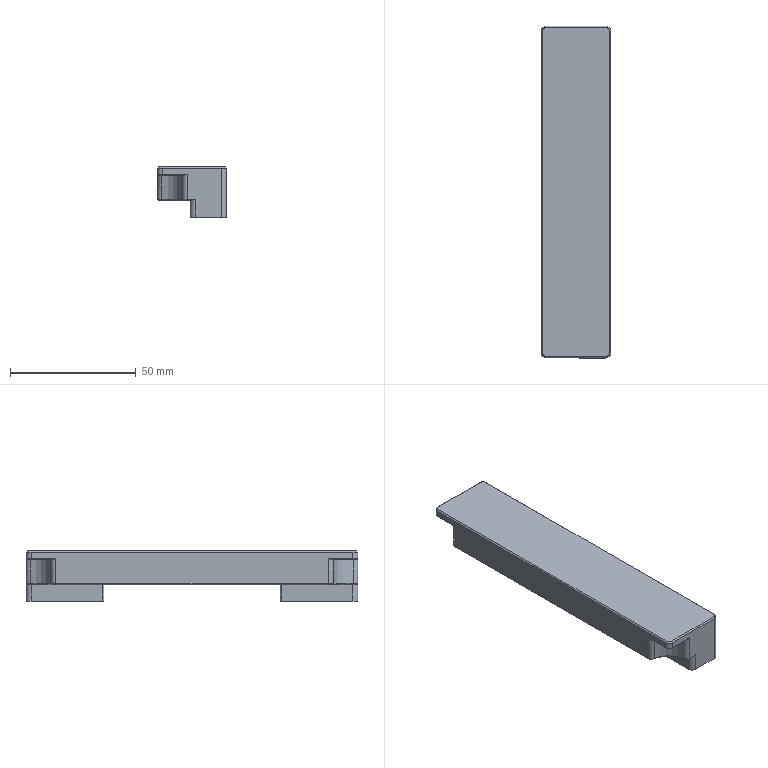NC program | NX | posted with a generic post | part box 27.5 x 132 x 20 mm
Lines 1924 to 2947 of 2947:
(ZLEVEL_PROFILE_COPY_1_COPY , TOOL : D10JING)
N3822 T14 M6
N3824 G54
N3826 G17 G0 G90 X45.895 Y-18.75 S9500 M3
N3828 G43 Z30. H14
N3830 Z1.5
N3832 G94 G1 X-64.649 Z-4.293 F1000.
N3834 X-66.234 Y-18.416 Z-4.378
N3836 X-67.701 Y-17.727 Z-4.463
N3838 X-68.971 Y-16.721 Z-4.548
N3840 X-69.977 Y-15.451 Z-4.633
N3842 X-70.666 Y-13.984 Z-4.718
N3844 X-71. Y-12.399 Z-4.803
N3846 Y12.399 Z-6.102
N3848 X-70.666 Y13.984 Z-6.187
N3850 X-69.977 Y15.451 Z-6.272
N3852 X-68.971 Y16.721 Z-6.357
N3854 X-67.701 Y17.727 Z-6.442
N3856 X-66.234 Y18.416 Z-6.527
N3858 X-64.649 Y18.75 Z-6.612
N3860 X0. Z-10.
N3862 X64. F1200.
N3864 G2 X71. Y11.75 R7.
N3866 G1 Y-11.75
N3868 G2 X64. Y-18.75 R7.
N3870 G1 X-64.
N3872 G2 X-71. Y-11.75 R7.
N3874 G1 Y11.75
N3876 G2 X-64. Y18.75 R7.
N3878 G1 X0.
N3880 X64. Z-11.845
N3882 X64.61 Y18.723 Z-11.862
N3884 X65.216 Y18.644 Z-11.88
N3886 X65.812 Y18.511 Z-11.898
N3888 X66.394 Y18.328 Z-11.915
N3890 X66.958 Y18.094 Z-11.933
N3892 X67.5 Y17.812 Z-11.95
N3894 X68.015 Y17.484 Z-11.968
N3896 X68.5 Y17.112 Z-11.985
N3898 X68.95 Y16.7 Z-12.003
N3900 X69.362 Y16.25 Z-12.021
N3902 X69.734 Y15.765 Z-12.038
N3904 X70.062 Y15.25 Z-12.056
N3906 X70.344 Y14.708 Z-12.073
N3908 X70.578 Y14.144 Z-12.091
N3910 X70.761 Y13.562 Z-12.109
N3912 X70.894 Y12.966 Z-12.126
N3914 X70.973 Y12.36 Z-12.144
N3916 X71. Y11.75 Z-12.161
N3918 Y-11.75 Z-12.839
N3920 X70.973 Y-12.36 Z-12.856
N3922 X70.894 Y-12.966 Z-12.874
N3924 X70.761 Y-13.562 Z-12.891
N3926 X70.578 Y-14.144 Z-12.909
N3928 X70.344 Y-14.708 Z-12.927
N3930 X70.062 Y-15.25 Z-12.944
N3932 X69.734 Y-15.765 Z-12.962
N3934 X69.362 Y-16.25 Z-12.979
N3936 X68.95 Y-16.7 Z-12.997
N3938 X68.5 Y-17.112 Z-13.015
N3940 X68.015 Y-17.484 Z-13.032
N3942 X67.5 Y-17.812 Z-13.05
N3944 X66.958 Y-18.094 Z-13.067
N3946 X66.394 Y-18.328 Z-13.085
N3948 X65.812 Y-18.511 Z-13.102
N3950 X65.216 Y-18.644 Z-13.12
N3952 X64.61 Y-18.723 Z-13.138
N3954 X64. Y-18.75 Z-13.155
N3956 X-64. Z-16.845
N3958 X-64.61 Y-18.723 Z-16.862
N3960 X-65.216 Y-18.644 Z-16.88
N3962 X-65.812 Y-18.511 Z-16.898
N3964 X-66.394 Y-18.328 Z-16.915
N3966 X-66.958 Y-18.094 Z-16.933
N3968 X-67.5 Y-17.812 Z-16.95
N3970 X-68.015 Y-17.484 Z-16.968
N3972 X-68.5 Y-17.112 Z-16.985
N3974 X-68.95 Y-16.7 Z-17.003
N3976 X-69.362 Y-16.25 Z-17.021
N3978 X-69.734 Y-15.765 Z-17.038
N3980 X-70.062 Y-15.25 Z-17.056
N3982 X-70.344 Y-14.708 Z-17.073
N3984 X-70.578 Y-14.144 Z-17.091
N3986 X-70.761 Y-13.562 Z-17.109
N3988 X-70.894 Y-12.966 Z-17.126
N3990 X-70.973 Y-12.36 Z-17.144
N3992 X-71. Y-11.75 Z-17.161
N3994 Y11.75 Z-17.839
N3996 X-70.973 Y12.36 Z-17.856
N3998 X-70.894 Y12.966 Z-17.874
N4000 X-70.761 Y13.562 Z-17.891
N4002 X-70.578 Y14.144 Z-17.909
N4004 X-70.344 Y14.708 Z-17.927
N4006 X-70.062 Y15.25 Z-17.944
N4008 X-69.734 Y15.765 Z-17.962
N4010 X-69.362 Y16.25 Z-17.979
N4012 X-68.95 Y16.7 Z-17.997
N4014 X-68.5 Y17.112 Z-18.015
N4016 X-68.015 Y17.484 Z-18.032
N4018 X-67.5 Y17.812 Z-18.05
N4020 X-66.958 Y18.094 Z-18.067
N4022 X-66.394 Y18.328 Z-18.085
N4024 X-65.812 Y18.511 Z-18.102
N4026 X-65.216 Y18.644 Z-18.12
N4028 X-64.61 Y18.723 Z-18.138
N4030 X-64. Y18.75 Z-18.155
N4032 X0. Z-20.
N4034 X64.
N4036 G2 X71. Y11.75 R7.
N4038 G1 Y-11.75
N4040 G2 X64. Y-18.75 R7.
N4042 G1 X-64.
N4044 G2 X-71. Y-11.75 R7.
N4046 G1 Y11.75
N4048 G2 X-64. Y18.75 R7.
N4050 G1 X0.
N4052 G3 X0.866 Y19.25 R1.
N4054 G1 X1.155 Y19.75
N4056 Z-19.
N4058 G0 Z30.
(FLOOR_WALL_2 , TOOL : D10JING)
N4060 X-73.846 Y-3.664
N4062 Z-13.5
N4064 G1 Z-16.5 F1500.
N4066 X-70.5 Y-5.715
N4068 X-70.45 Y-5.746
N4070 G3 X-65.25 Y-9.313 R7.5
N4072 G2 X-63.649 Y-9.913 R4.5
N4074 G1 X-63.648 Z-13.5
N4076 G0 Z30.
N4078 X-54.067 Y-21.75
N4080 Z-13.5
N4082 G1 Z-16.5
N4084 Y-19.365
N4086 X-56.84 Y-18.22
N4088 G2 X-61.07 Y-12.917 R7.
N4090 G3 X-65.167 Y-8.82 R5.
N4092 G2 X-70.47 Y-4.59 R7.
N4094 G1 X-71.615 Y-1.817
N4096 X-74.
N4098 Z-13.5
N4100 G0 Z30.
N4102 X-27. Y7.25
N4104 Z-3.5
N4106 G1 Z-6.5
N4108 X-29.5 Y4.25
N4110 X29.5
N4112 Y-0.25
N4114 X-29.5
N4116 Y-2.321
N4118 G2 X-29.646 Y-2.675 R0.5
N4120 G1 X-31.722 Y-4.75
N4122 X31.722
N4124 X33.075 Y-6.104
N4126 G3 X33.429 Y-6.25 R0.5
N4128 G1 X64.
N4130 G3 X68.5 Y-4.75 R7.5
N4132 G1 X69.851
N4134 X73.068
N4136 Z-3.5
N4138 G0 Z30.
N4140 X-73.068
N4142 Z-3.5
N4144 G1 Z-6.5
N4146 X-69.851
N4148 X-68.5
N4150 X-72.04 Y-6.978
N4152 Z-3.5
N4154 G0 Z30.
N4156 X70.041 Y-9.25
N4158 Z-3.5
N4160 G1 Z-6.5
N4162 X62.838
N4164 X-62.838
N4166 X-70.041
N4168 Z-3.5
N4170 G0 Z30.
N4172 X-27. Y7.25
N4174 Z-3.5
N4176 G1 Z-6.5
N4178 X-30.
N4180 Y4.25
N4182 Y-2.321
N4184 X-33.429 Y-5.75
N4186 X-64.
N4188 G2 X-70.47 Y-1.422 R7.
N4190 G1 X-71.615 Y1.351
N4192 X-74.
N4194 Z-3.5
N4196 G0 Z30.
N4198 X74.
N4200 Z-3.5
N4202 G1 Z-6.5
N4204 X71.615
N4206 X70.47 Y-1.422
N4208 G2 X64. Y-5.75 R7.
N4210 G1 X33.429
N4212 X30. Y-2.321
N4214 Y4.25
N4216 Y7.25
N4218 X27.
N4220 Z-3.5
N4222 G0 Z30.
N4224 X-34.307 Y21.75
N4226 Z-13.5
N4228 G1 Z-16.5
N4230 Y18.75
N4232 X34.307
N4234 G3 X29.872 Y14.083 R7.5
N4236 G1 X-29.872
N4238 G2 X-29.5 Y11.75 R7.5
N4240 G1 Y9.417
N4242 X29.5
N4244 Y4.75
N4246 X-29.5
N4248 Z-13.5
N4250 G0 Z30.
N4252 X-39.34 Y21.75
N4254 Z-13.5
N4256 G1 Z-16.5
N4258 Y18.997
N4260 X-36.353 Y18.72
N4262 G2 X-30. Y11.75 R7.
N4264 G1 Y4.25
N4266 X30.
N4268 Y11.75
N4270 G2 X36.353 Y18.72 R7.
N4272 G1 X39.34 Y18.997
N4274 Y21.75
N4276 Z-13.5
N4278 G0 Z30.
N4280 X73.5 Y-8.364
N4282 Z-13.5
N4284 G1 Z-16.5
N4286 X67.834
N4288 X61.776 Y-18.25
N4290 X57.965
N4292 X57.996 Y-18.2
N4294 Y-21.25
N4296 Z-13.5
N4298 G0 Z30.
N4300 Y-18.2
N4302 Z-13.5
N4304 G1 Z-16.5
N4306 G3 X61.563 Y-13. R7.5
N4308 G2 X62.16 Y-11.404 R4.5
N4310 G1 X62.166 Y-11.394
N4312 Z-13.5
N4314 G0 Z30.
N4316 X74. Y-1.817
N4318 Z-13.5
N4320 G1 Z-16.5
N4322 X71.615
N4324 X70.47 Y-4.59
N4326 G2 X65.167 Y-8.82 R7.
N4328 G3 X61.07 Y-12.917 R5.
N4330 G2 X56.84 Y-18.22 R7.
N4332 G1 X54.067 Y-19.365
N4334 Y-21.75
N4336 Z-13.5
N4338 G0 Z30.
N4340 M5
(HOLE_MILLING , TOOL : D4)
N4342 T11 M6
N4344 G54
N4346 G17 G0 G90 X-60. Y8.75 S9500 M3
N4348 G43 Z30. H11
N4350 Z0.5
N4352 G94 G3 X-59.5 Y9.25 R0.5 F1250.
N4354 X-60. Y9.75 R0.5
N4356 X-60. Y9.75 Z0.1 I0. J-1.
N4358 X-60. Y9.75 Z-0.3 I0. J-1.
N4360 X-60. Y9.75 Z-0.7 I0. J-1.
N4362 X-60. Y9.75 Z-1.1 I0. J-1.
N4364 X-60. Y9.75 Z-1.5 I0. J-1.
N4366 X-60. Y9.75 Z-1.9 I0. J-1.
N4368 X-60. Y9.75 Z-2.3 I0. J-1.
N4370 X-60. Y9.75 Z-2.7 I0. J-1.
N4372 X-60. Y9.75 Z-3.1 I0. J-1.
N4374 X-60. Y9.75 Z-3.5 I0. J-1.
N4376 X-60. Y9.75 Z-3.9 I0. J-1.
N4378 X-60. Y9.75 Z-4.3 I0. J-1.
N4380 X-60. Y9.75 Z-4.7 I0. J-1.
N4382 X-60. Y9.75 Z-5.1 I0. J-1.
N4384 X-60. Y9.75 Z-5.5 I0. J-1.
N4386 X-60. Y9.75 Z-5.9 I0. J-1.
N4388 X-60. Y9.75 Z-6.3 I0. J-1.
N4390 X-60. Y9.75 Z-6.7 I0. J-1.
N4392 X-60. Y9.75 Z-7.1 I0. J-1.
N4394 X-60. Y9.75 Z-7.5 I0. J-1.
N4396 X-60. Y9.75 Z-7.9 I0. J-1.
N4398 X-60. Y9.75 Z-8.3 I0. J-1.
N4400 X-60. Y9.75 Z-8.7 I0. J-1.
N4402 X-60. Y9.75 Z-9.1 I0. J-1.
N4404 X-60. Y9.75 Z-9.5 I0. J-1.
N4406 X-60. Y9.75 Z-9.9 I0. J-1.
N4408 X-60. Y9.75 Z-10.3 I0. J-1.
N4410 X-60. Y9.75 Z-10.7 I0. J-1.
N4412 X-60. Y9.75 Z-11.1 I0. J-1.
N4414 X-60. Y9.75 Z-11.5 I0. J-1.
N4416 X-60. Y9.75 Z-11.9 I0. J-1.
N4418 X-61. Y8.75 Z-12. R1.
N4420 X-60. Y7.75 R1.
N4422 X-61. Y8.75 R-1.
N4424 X-60.5 Y8.25 R0.5
N4426 X-60. Y8.75 R0.5
N4428 G0 Z30.
N4430 X-37.5 Y-8.75
N4432 Z-6.
N4434 G3 X-37. Y-8.25 R0.5
N4436 X-37.5 Y-7.75 R0.5
N4438 X-37.5 Y-7.75 Z-6.4 I0. J-1.
N4440 X-37.5 Y-7.75 Z-6.8 I0. J-1.
N4442 X-37.5 Y-7.75 Z-7.2 I0. J-1.
N4444 X-37.5 Y-7.75 Z-7.6 I0. J-1.
N4446 X-37.5 Y-7.75 Z-8. I0. J-1.
N4448 X-37.5 Y-7.75 Z-8.4 I0. J-1.
N4450 X-37.5 Y-7.75 Z-8.8 I0. J-1.
N4452 X-37.5 Y-7.75 Z-9.2 I0. J-1.
N4454 X-37.5 Y-7.75 Z-9.6 I0. J-1.
N4456 X-37.5 Y-7.75 Z-10. I0. J-1.
N4458 X-37.5 Y-7.75 Z-10.4 I0. J-1.
N4460 X-37.5 Y-7.75 Z-10.8 I0. J-1.
N4462 X-37.5 Y-7.75 Z-11.2 I0. J-1.
N4464 X-37.5 Y-7.75 Z-11.6 I0. J-1.
N4466 X-37.5 Y-7.75 Z-12. I0. J-1.
N4468 X-37.5 Y-7.75 Z-12.4 I0. J-1.
N4470 X-37.5 Y-7.75 Z-12.8 I0. J-1.
N4472 X-37.5 Y-7.75 Z-13.2 I0. J-1.
N4474 X-37.5 Y-7.75 Z-13.6 I0. J-1.
N4476 X-37.5 Y-7.75 Z-14. I0. J-1.
N4478 X-37.5 Y-7.75 Z-14.4 I0. J-1.
N4480 X-37.5 Y-7.75 Z-14.8 I0. J-1.
N4482 X-37.5 Y-7.75 Z-15.2 I0. J-1.
N4484 X-37.5 Y-7.75 Z-15.6 I0. J-1.
N4486 X-37.5 Y-7.75 Z-16. I0. J-1.
N4488 X-37.5 Y-7.75 Z-16.4 I0. J-1.
N4490 X-37.5 Y-7.75 Z-16.8 I0. J-1.
N4492 X-37.5 Y-9.75 Z-17. I0. J-1.
N4494 X-36.5 Y-8.75 R1.
N4496 X-37.5 Y-9.75 R-1.
N4498 X-37. Y-9.25 R0.5
N4500 X-37.5 Y-8.75 R0.5
N4502 G0 Z30.
N4504 X37.5
N4506 Z-6.
N4508 G3 X38. Y-8.25 R0.5
N4510 X37.5 Y-7.75 R0.5
N4512 X37.5 Y-7.75 Z-6.4 I0. J-1.
N4514 X37.5 Y-7.75 Z-6.8 I0. J-1.
N4516 X37.5 Y-7.75 Z-7.2 I0. J-1.
N4518 X37.5 Y-7.75 Z-7.6 I0. J-1.
N4520 X37.5 Y-7.75 Z-8. I0. J-1.
N4522 X37.5 Y-7.75 Z-8.4 I0. J-1.
N4524 X37.5 Y-7.75 Z-8.8 I0. J-1.
N4526 X37.5 Y-7.75 Z-9.2 I0. J-1.
N4528 X37.5 Y-7.75 Z-9.6 I0. J-1.
N4530 X37.5 Y-7.75 Z-10. I0. J-1.
N4532 X37.5 Y-7.75 Z-10.4 I0. J-1.
N4534 X37.5 Y-7.75 Z-10.8 I0. J-1.
N4536 X37.5 Y-7.75 Z-11.2 I0. J-1.
N4538 X37.5 Y-7.75 Z-11.6 I0. J-1.
N4540 X37.5 Y-7.75 Z-12. I0. J-1.
N4542 X37.5 Y-7.75 Z-12.4 I0. J-1.
N4544 X37.5 Y-7.75 Z-12.8 I0. J-1.
N4546 X37.5 Y-7.75 Z-13.2 I0. J-1.
N4548 X37.5 Y-7.75 Z-13.6 I0. J-1.
N4550 X37.5 Y-7.75 Z-14. I0. J-1.
N4552 X37.5 Y-7.75 Z-14.4 I0. J-1.
N4554 X37.5 Y-7.75 Z-14.8 I0. J-1.
N4556 X37.5 Y-7.75 Z-15.2 I0. J-1.
N4558 X37.5 Y-7.75 Z-15.6 I0. J-1.
N4560 X37.5 Y-7.75 Z-16. I0. J-1.
N4562 X37.5 Y-7.75 Z-16.4 I0. J-1.
N4564 X37.5 Y-7.75 Z-16.8 I0. J-1.
N4566 X37.5 Y-9.75 Z-17. I0. J-1.
N4568 X38.5 Y-8.75 R1.
N4570 X37.5 Y-9.75 R-1.
N4572 X38. Y-9.25 R0.5
N4574 X37.5 Y-8.75 R0.5
N4576 G0 Z30.
N4578 X60. Y8.75
N4580 Z0.5
N4582 G3 X60.5 Y9.25 R0.5
N4584 X60. Y9.75 R0.5
N4586 X60. Y9.75 Z0.1 I0. J-1.
N4588 X60. Y9.75 Z-0.3 I0. J-1.
N4590 X60. Y9.75 Z-0.7 I0. J-1.
N4592 X60. Y9.75 Z-1.1 I0. J-1.
N4594 X60. Y9.75 Z-1.5 I0. J-1.
N4596 X60. Y9.75 Z-1.9 I0. J-1.
N4598 X60. Y9.75 Z-2.3 I0. J-1.
N4600 X60. Y9.75 Z-2.7 I0. J-1.
N4602 X60. Y9.75 Z-3.1 I0. J-1.
N4604 X60. Y9.75 Z-3.5 I0. J-1.
N4606 X60. Y9.75 Z-3.9 I0. J-1.
N4608 X60. Y9.75 Z-4.3 I0. J-1.
N4610 X60. Y9.75 Z-4.7 I0. J-1.
N4612 X60. Y9.75 Z-5.1 I0. J-1.
N4614 X60. Y9.75 Z-5.5 I0. J-1.
N4616 X60. Y9.75 Z-5.9 I0. J-1.
N4618 X60. Y9.75 Z-6.3 I0. J-1.
N4620 X60. Y9.75 Z-6.7 I0. J-1.
N4622 X60. Y9.75 Z-7.1 I0. J-1.
N4624 X60. Y9.75 Z-7.5 I0. J-1.
N4626 X60. Y9.75 Z-7.9 I0. J-1.
N4628 X60. Y9.75 Z-8.3 I0. J-1.
N4630 X60. Y9.75 Z-8.7 I0. J-1.
N4632 X60. Y9.75 Z-9.1 I0. J-1.
N4634 X60. Y9.75 Z-9.5 I0. J-1.
N4636 X60. Y9.75 Z-9.9 I0. J-1.
N4638 X60. Y9.75 Z-10.3 I0. J-1.
N4640 X60. Y9.75 Z-10.7 I0. J-1.
N4642 X60. Y9.75 Z-11.1 I0. J-1.
N4644 X60. Y9.75 Z-11.5 I0. J-1.
N4646 X60. Y9.75 Z-11.9 I0. J-1.
N4648 X59. Y8.75 Z-12. R1.
N4650 X60. Y7.75 R1.
N4652 X59. Y8.75 R-1.
N4654 X59.5 Y8.25 R0.5
N4656 X60. Y8.75 R0.5
N4658 G0 Z30.
(ZLEVEL_PROFILE_COPY_1_COPY_1 , TOOL : D4)
N4660 X-32.6 Y4.609
N4662 Z-6.9
N4664 G1 X-32.8 Y4.493 F1000.
N4666 G3 X-33. Y4.147 R0.4
N4668 G1 Y1.25 F1800.
N4670 X-30.103
N4672 G3 X-29.757 Y1.45 R0.4
N4674 G1 X-29.641 Y1.65
N4676 G0 X-32.6 Y4.609 Z-7.3
N4678 G1 X-32.8 Y4.493 F1000.
N4680 G3 X-33. Y4.147 R0.4
N4682 G1 Y1.25 F1800.
N4684 X-30.103
N4686 G3 X-29.757 Y1.45 R0.4
N4688 G1 X-29.641 Y1.65
N4690 G0 X-32.6 Y4.609 Z-7.7
N4692 G1 X-32.8 Y4.493 F1000.
N4694 G3 X-33. Y4.147 R0.4
N4696 G1 Y1.25 F1800.
N4698 X-30.103
N4700 G3 X-29.757 Y1.45 R0.4
N4702 G1 X-29.641 Y1.65
N4704 G0 X-32.6 Y4.609 Z-8.1
N4706 G1 X-32.8 Y4.493 F1000.
N4708 G3 X-33. Y4.147 R0.4
N4710 G1 Y1.25 F1800.
N4712 X-30.103
N4714 G3 X-29.757 Y1.45 R0.4
N4716 G1 X-29.641 Y1.65
N4718 G0 X-32.6 Y4.609 Z-8.5
N4720 G1 X-32.8 Y4.493 F1000.
N4722 G3 X-33. Y4.147 R0.4
N4724 G1 Y1.25 F1800.
N4726 X-30.103
N4728 G3 X-29.757 Y1.45 R0.4
N4730 G1 X-29.641 Y1.65
N4732 G0 X-32.6 Y4.609 Z-8.9
N4734 G1 X-32.8 Y4.493 F1000.
N4736 G3 X-33. Y4.147 R0.4
N4738 G1 Y1.25 F1800.
N4740 X-30.103
N4742 G3 X-29.757 Y1.45 R0.4
N4744 G1 X-29.641 Y1.65
N4746 G0 X-32.6 Y4.609 Z-9.3
N4748 G1 X-32.8 Y4.493 F1000.
N4750 G3 X-33. Y4.147 R0.4
N4752 G1 Y1.25 F1800.
N4754 X-30.103
N4756 G3 X-29.757 Y1.45 R0.4
N4758 G1 X-29.641 Y1.65
N4760 G0 X-32.6 Y4.609 Z-9.7
N4762 G1 X-32.8 Y4.493 F1000.
N4764 G3 X-33. Y4.147 R0.4
N4766 G1 Y1.25 F1800.
N4768 X-30.103
N4770 G3 X-29.757 Y1.45 R0.4
N4772 G1 X-29.641 Y1.65
N4774 G0 X-32.6 Y4.609 Z-10.1
N4776 G1 X-32.8 Y4.493 F1000.
N4778 G3 X-33. Y4.147 R0.4
N4780 G1 Y1.25 F1800.
N4782 X-30.103
N4784 G3 X-29.757 Y1.45 R0.4
N4786 G1 X-29.641 Y1.65
N4788 G0 X-32.6 Y4.609 Z-10.5
N4790 G1 X-32.8 Y4.493 F1000.
N4792 G3 X-33. Y4.147 R0.4
N4794 G1 Y1.25 F1800.
N4796 X-30.103
N4798 G3 X-29.757 Y1.45 R0.4
N4800 G1 X-29.641 Y1.65
N4802 G0 X-32.6 Y4.609 Z-10.9
N4804 G1 X-32.8 Y4.493 F1000.
N4806 G3 X-33. Y4.147 R0.4
N4808 G1 Y1.25 F1800.
N4810 X-30.103
N4812 G3 X-29.757 Y1.45 R0.4
N4814 G1 X-29.641 Y1.65
N4816 G0 X-32.6 Y4.609 Z-11.3
N4818 G1 X-32.8 Y4.493 F1000.
N4820 G3 X-33. Y4.147 R0.4
N4822 G1 Y1.25 F1800.
N4824 X-30.103
N4826 G3 X-29.757 Y1.45 R0.4
N4828 G1 X-29.641 Y1.65
N4830 G0 X-32.6 Y4.609 Z-11.7
N4832 G1 X-32.8 Y4.493 F1000.
N4834 G3 X-33. Y4.147 R0.4
N4836 G1 Y1.25 F1800.
N4838 X-30.103
N4840 G3 X-29.757 Y1.45 R0.4
N4842 G1 X-29.641 Y1.65
N4844 G0 X-32.6 Y4.609 Z-12.1
N4846 G1 X-32.8 Y4.493 F1000.
N4848 G3 X-33. Y4.147 R0.4
N4850 G1 Y1.25 F1800.
N4852 X-30.103
N4854 G3 X-29.757 Y1.45 R0.4
N4856 G1 X-29.641 Y1.65
N4858 G0 X-32.6 Y4.609 Z-12.5
N4860 G1 X-32.8 Y4.493 F1000.
N4862 G3 X-33. Y4.147 R0.4
N4864 G1 Y1.25 F1800.
N4866 X-30.103
N4868 G3 X-29.757 Y1.45 R0.4
N4870 G1 X-29.641 Y1.65
N4872 G0 X-32.6 Y4.609 Z-12.9
N4874 G1 X-32.8 Y4.493 F1000.
N4876 G3 X-33. Y4.147 R0.4
N4878 G1 Y1.25 F1800.
N4880 X-30.103
N4882 G3 X-29.757 Y1.45 R0.4
N4884 G1 X-29.641 Y1.65
N4886 G0 X-32.6 Y4.609 Z-13.3
N4888 G1 X-32.8 Y4.493 F1000.
N4890 G3 X-33. Y4.147 R0.4
N4892 G1 Y1.25 F1800.
N4894 X-30.103
N4896 G3 X-29.757 Y1.45 R0.4
N4898 G1 X-29.641 Y1.65
N4900 G0 X-32.6 Y4.609 Z-13.7
N4902 G1 X-32.8 Y4.493 F1000.
N4904 G3 X-33. Y4.147 R0.4
N4906 G1 Y1.25 F1800.
N4908 X-30.103
N4910 G3 X-29.757 Y1.45 R0.4
N4912 G1 X-29.641 Y1.65
N4914 G0 X-32.6 Y4.609 Z-14.1
N4916 G1 X-32.8 Y4.493 F1000.
N4918 G3 X-33. Y4.147 R0.4
N4920 G1 Y1.25 F1800.
N4922 X-30.103
N4924 G3 X-29.757 Y1.45 R0.4
N4926 G1 X-29.641 Y1.65
N4928 G0 X-32.6 Y4.609 Z-14.5
N4930 G1 X-32.8 Y4.493 F1000.
N4932 G3 X-33. Y4.147 R0.4
N4934 G1 Y1.25 F1800.
N4936 X-30.103
N4938 G3 X-29.757 Y1.45 R0.4
N4940 G1 X-29.641 Y1.65
N4942 G0 X-32.6 Y4.609 Z-14.9
N4944 G1 X-32.8 Y4.493 F1000.
N4946 G3 X-33. Y4.147 R0.4
N4948 G1 Y1.25 F1800.
N4950 X-30.103
N4952 G3 X-29.757 Y1.45 R0.4
N4954 G1 X-29.641 Y1.65
N4956 G0 X-32.6 Y4.609 Z-15.3
N4958 G1 X-32.8 Y4.493 F1000.
N4960 G3 X-33. Y4.147 R0.4
N4962 G1 Y1.25 F1800.
N4964 X-30.103
N4966 G3 X-29.757 Y1.45 R0.4
N4968 G1 X-29.641 Y1.65
N4970 G0 X-32.6 Y4.609 Z-15.7
N4972 G1 X-32.8 Y4.493 F1000.
N4974 G3 X-33. Y4.147 R0.4
N4976 G1 Y1.25 F1800.
N4978 X-30.103
N4980 G3 X-29.757 Y1.45 R0.4
N4982 G1 X-29.641 Y1.65
N4984 G0 X-32.6 Y4.609 Z-16.1
N4986 G1 X-32.8 Y4.493 F1000.
N4988 G3 X-33. Y4.147 R0.4
N4990 G1 Y1.25 F1800.
N4992 X-30.103
N4994 G3 X-29.757 Y1.45 R0.4
N4996 G1 X-29.641 Y1.65
N4998 G0 X-32.6 Y4.609 Z-16.5
N5000 G1 X-32.8 Y4.493 F1000.
N5002 G3 X-33. Y4.147 R0.4
N5004 G1 Y1.25 F1800.
N5006 X-30.103
N5008 G3 X-29.757 Y1.45 R0.4
N5010 G1 X-29.641 Y1.65
N5012 G0 Z30.
N5014 X29.641
N5016 Z-6.9
N5018 G1 X29.757 Y1.45 F1000.
N5020 G3 X30.103 Y1.25 R0.4
N5022 G1 X33. F1800.
N5024 Y4.147
N5026 G3 X32.8 Y4.493 R0.4
N5028 G1 X32.6 Y4.609
N5030 G0 X29.641 Y1.65 Z-7.3
N5032 G1 X29.757 Y1.45 F1000.
N5034 G3 X30.103 Y1.25 R0.4
N5036 G1 X33. F1800.
N5038 Y4.147
N5040 G3 X32.8 Y4.493 R0.4
N5042 G1 X32.6 Y4.609
N5044 G0 X29.641 Y1.65 Z-7.7
N5046 G1 X29.757 Y1.45 F1000.
N5048 G3 X30.103 Y1.25 R0.4
N5050 G1 X33. F1800.
N5052 Y4.147
N5054 G3 X32.8 Y4.493 R0.4
N5056 G1 X32.6 Y4.609
N5058 G0 X29.641 Y1.65 Z-8.1
N5060 G1 X29.757 Y1.45 F1000.
N5062 G3 X30.103 Y1.25 R0.4
N5064 G1 X33. F1800.
N5066 Y4.147
N5068 G3 X32.8 Y4.493 R0.4
N5070 G1 X32.6 Y4.609
N5072 G0 X29.641 Y1.65 Z-8.5
N5074 G1 X29.757 Y1.45 F1000.
N5076 G3 X30.103 Y1.25 R0.4
N5078 G1 X33. F1800.
N5080 Y4.147
N5082 G3 X32.8 Y4.493 R0.4
N5084 G1 X32.6 Y4.609
N5086 G0 X29.641 Y1.65 Z-8.9
N5088 G1 X29.757 Y1.45 F1000.
N5090 G3 X30.103 Y1.25 R0.4
N5092 G1 X33. F1800.
N5094 Y4.147
N5096 G3 X32.8 Y4.493 R0.4
N5098 G1 X32.6 Y4.609
N5100 G0 X29.641 Y1.65 Z-9.3
N5102 G1 X29.757 Y1.45 F1000.
N5104 G3 X30.103 Y1.25 R0.4
N5106 G1 X33. F1800.
N5108 Y4.147
N5110 G3 X32.8 Y4.493 R0.4
N5112 G1 X32.6 Y4.609
N5114 G0 X29.641 Y1.65 Z-9.7
N5116 G1 X29.757 Y1.45 F1000.
N5118 G3 X30.103 Y1.25 R0.4
N5120 G1 X33. F1800.
N5122 Y4.147
N5124 G3 X32.8 Y4.493 R0.4
N5126 G1 X32.6 Y4.609
N5128 G0 X29.641 Y1.65 Z-10.1
N5130 G1 X29.757 Y1.45 F1000.
N5132 G3 X30.103 Y1.25 R0.4
N5134 G1 X33. F1800.
N5136 Y4.147
N5138 G3 X32.8 Y4.493 R0.4
N5140 G1 X32.6 Y4.609
N5142 G0 X29.641 Y1.65 Z-10.5
N5144 G1 X29.757 Y1.45 F1000.
N5146 G3 X30.103 Y1.25 R0.4
N5148 G1 X33. F1800.
N5150 Y4.147
N5152 G3 X32.8 Y4.493 R0.4
N5154 G1 X32.6 Y4.609
N5156 G0 X29.641 Y1.65 Z-10.9
N5158 G1 X29.757 Y1.45 F1000.
N5160 G3 X30.103 Y1.25 R0.4
N5162 G1 X33. F1800.
N5164 Y4.147
N5166 G3 X32.8 Y4.493 R0.4
N5168 G1 X32.6 Y4.609
N5170 G0 X29.641 Y1.65 Z-11.3
N5172 G1 X29.757 Y1.45 F1000.
N5174 G3 X30.103 Y1.25 R0.4
N5176 G1 X33. F1800.
N5178 Y4.147
N5180 G3 X32.8 Y4.493 R0.4
N5182 G1 X32.6 Y4.609
N5184 G0 X29.641 Y1.65 Z-11.7
N5186 G1 X29.757 Y1.45 F1000.
N5188 G3 X30.103 Y1.25 R0.4
N5190 G1 X33. F1800.
N5192 Y4.147
N5194 G3 X32.8 Y4.493 R0.4
N5196 G1 X32.6 Y4.609
N5198 G0 X29.641 Y1.65 Z-12.1
N5200 G1 X29.757 Y1.45 F1000.
N5202 G3 X30.103 Y1.25 R0.4
N5204 G1 X33. F1800.
N5206 Y4.147
N5208 G3 X32.8 Y4.493 R0.4
N5210 G1 X32.6 Y4.609
N5212 G0 X29.641 Y1.65 Z-12.5
N5214 G1 X29.757 Y1.45 F1000.
N5216 G3 X30.103 Y1.25 R0.4
N5218 G1 X33. F1800.
N5220 Y4.147
N5222 G3 X32.8 Y4.493 R0.4
N5224 G1 X32.6 Y4.609
N5226 G0 X29.641 Y1.65 Z-12.9
N5228 G1 X29.757 Y1.45 F1000.
N5230 G3 X30.103 Y1.25 R0.4
N5232 G1 X33. F1800.
N5234 Y4.147
N5236 G3 X32.8 Y4.493 R0.4
N5238 G1 X32.6 Y4.609
N5240 G0 X29.641 Y1.65 Z-13.3
N5242 G1 X29.757 Y1.45 F1000.
N5244 G3 X30.103 Y1.25 R0.4
N5246 G1 X33. F1800.
N5248 Y4.147
N5250 G3 X32.8 Y4.493 R0.4
N5252 G1 X32.6 Y4.609
N5254 G0 X29.641 Y1.65 Z-13.7
N5256 G1 X29.757 Y1.45 F1000.
N5258 G3 X30.103 Y1.25 R0.4
N5260 G1 X33. F1800.
N5262 Y4.147
N5264 G3 X32.8 Y4.493 R0.4
N5266 G1 X32.6 Y4.609
N5268 G0 X29.641 Y1.65 Z-14.1
N5270 G1 X29.757 Y1.45 F1000.
N5272 G3 X30.103 Y1.25 R0.4
N5274 G1 X33. F1800.
N5276 Y4.147
N5278 G3 X32.8 Y4.493 R0.4
N5280 G1 X32.6 Y4.609
N5282 G0 X29.641 Y1.65 Z-14.5
N5284 G1 X29.757 Y1.45 F1000.
N5286 G3 X30.103 Y1.25 R0.4
N5288 G1 X33. F1800.
N5290 Y4.147
N5292 G3 X32.8 Y4.493 R0.4
N5294 G1 X32.6 Y4.609
N5296 G0 X29.641 Y1.65 Z-14.9
N5298 G1 X29.757 Y1.45 F1000.
N5300 G3 X30.103 Y1.25 R0.4
N5302 G1 X33. F1800.
N5304 Y4.147
N5306 G3 X32.8 Y4.493 R0.4
N5308 G1 X32.6 Y4.609
N5310 G0 X29.641 Y1.65 Z-15.3
N5312 G1 X29.757 Y1.45 F1000.
N5314 G3 X30.103 Y1.25 R0.4
N5316 G1 X33. F1800.
N5318 Y4.147
N5320 G3 X32.8 Y4.493 R0.4
N5322 G1 X32.6 Y4.609
N5324 G0 X29.641 Y1.65 Z-15.7
N5326 G1 X29.757 Y1.45 F1000.
N5328 G3 X30.103 Y1.25 R0.4
N5330 G1 X33. F1800.
N5332 Y4.147
N5334 G3 X32.8 Y4.493 R0.4
N5336 G1 X32.6 Y4.609
N5338 G0 X29.641 Y1.65 Z-16.1
N5340 G1 X29.757 Y1.45 F1000.
N5342 G3 X30.103 Y1.25 R0.4
N5344 G1 X33. F1800.
N5346 Y4.147
N5348 G3 X32.8 Y4.493 R0.4
N5350 G1 X32.6 Y4.609
N5352 G0 X29.641 Y1.65 Z-16.5
N5354 G1 X29.757 Y1.45 F1000.
N5356 G3 X30.103 Y1.25 R0.4
N5358 G1 X33. F1800.
N5360 Y4.147
N5362 G3 X32.8 Y4.493 R0.4
N5364 G1 X32.6 Y4.609
N5366 G0 Z30.
N5368 M5
(PLANAR_MILL_COPY_COPY_COPY_COPY_COPY_COPY_COPY_COPY_1 , TOOL : D6A45)
N5370 T01 M6
N5372 G54
N5374 G17 G0 G90 X51.041 Y-3.35 S9500 M3
N5376 G43 Z30. H1
N5378 Z0.
N5380 G94 G1 Z-1.5 F1250.
N5382 X50.637 Y-2.65
N5384 G3 X49.771 Y-2.15 R1.
N5386 G1 X35.541
N5388 G2 X34.481 Y-1.711 R1.5
N5390 G1 X34.039 Y-1.269
N5392 G2 X33.6 Y-0.209 R1.5
N5394 G1 Y11.75
N5396 G2 X37. Y15.15 R3.4
N5398 G1 X64.
N5400 G2 X67.4 Y11.75 R3.4
N5402 G1 Y1.25
N5404 G2 X64. Y-2.15 R3.4
N5406 G1 X49.771
N5408 G3 X48.905 Y-2.65 R1.
N5410 G1 X48.501 Y-3.35
N5412 Z0.
N5414 G0 Z30.
N5416 X-48.501
N5418 Z0.
N5420 G1 Z-1.5
N5422 X-48.905 Y-2.65
N5424 G3 X-49.771 Y-2.15 R1.
N5426 G1 X-64.
N5428 G2 X-67.4 Y1.25 R3.4
N5430 G1 Y11.75
N5432 G2 X-64. Y15.15 R3.4
N5434 G1 X-37.
N5436 G2 X-33.6 Y11.75 R3.4
N5438 G1 Y-0.209
N5440 G2 X-34.039 Y-1.269 R1.5
N5442 G1 X-34.481 Y-1.711
N5444 G2 X-35.541 Y-2.15 R1.5
N5446 G1 X-49.771
N5448 G3 X-50.637 Y-2.65 R1.
N5450 G1 X-51.041 Y-3.35
N5452 Z0.
N5454 G0 Z30.
(PLANAR_MILL_COPY_COPY_COPY_COPY , TOOL : D6A45)
N5456 X60.517 Y9.943
N5458 Z0.
N5460 G1 Z-1.5
N5462 X60.866 Y10.75
N5464 G3 X60. Y11.25 R1.
N5466 X57.5 Y8.75 R2.5
N5468 X60. Y11.25 R-2.5
N5470 X59.134 Y10.75 R1.
N5472 G1 X59.483 Y9.943
N5474 Z0.
N5476 G0 Z30.
N5478 X-59.483
N5480 Z0.
N5482 G1 Z-1.5
N5484 X-59.134 Y10.75
N5486 G3 X-60. Y11.25 R1.
N5488 X-62.5 Y8.75 R2.5
N5490 X-60. Y11.25 R-2.5
N5492 X-60.866 Y10.75 R1.
N5494 G1 X-60.517 Y9.943
N5496 Z0.
N5498 G0 Z30.
(PLANAR_MILL_COPY_COPY_COPY_COPY_COPY , TOOL : D6A45)
N5500 X36.307 Y-8.233
N5502 Z-6.5
N5504 G1 Z-8.
N5506 X35.5 Y-7.884
N5508 G3 X35. Y-8.75 R1.
N5510 X37.5 Y-11.25 R2.5
N5512 X35. Y-8.75 R-2.5
N5514 X35.5 Y-9.616 R1.
N5516 G1 X36.307 Y-9.267
N5518 Z-6.5
N5520 G0 Z30.
N5522 X61.461 Y-5.995
N5524 Z-6.5
N5526 G1 X61.962 Y-5.673 Z-6.66
N5528 X63.775 Y-4.998 Z-7.178
N5530 X64.5 Y-4.876 Z-7.375
N5532 X64.919 Y-4.805 Z-7.489
N5534 X65.593 Y-4.495 Z-7.687
N5536 X66.171 Y-4.031 Z-7.886
N5538 X66.422 Y-3.688 Z-8.
N5540 G2 X64.5 Y-4.876 R3.
N5542 G3 X57.126 Y-12.25 R9.
N5544 G2 X54.168 Y-14.75 R3.
N5546 G1 X-54.168
N5548 G2 X-57.126 Y-12.25 R3.
N5550 G3 X-64.5 Y-4.876 R9.
N5552 G2 X-66.422 Y-3.688 R3.
N5554 G1 Z-6.5
N5556 G0 Z30.
N5558 X-38.693 Y-8.233
N5560 Z-6.5
N5562 G1 Z-8.
N5564 X-39.5 Y-7.884
N5566 G3 X-40. Y-8.75 R1.
N5568 X-37.5 Y-11.25 R2.5
N5570 X-40. Y-8.75 R-2.5
N5572 X-39.5 Y-9.616 R1.
N5574 G1 X-38.693 Y-9.267
N5576 Z-6.5
N5578 G0 Z30.
(PLANAR_MILL_COPY_COPY_COPY_COPY_COPY_COPY , TOOL : D6A45)
N5580 X68.606 Y-6.783
N5582 Z-16.5
N5584 G1 Z-18.
N5586 X67.999 Y-6.474
N5588 G3 X67. Y-6.528 R1.
N5590 G1 Y-11.75
N5592 G2 X64. Y-14.75 R3.
N5594 G1 X58.778
N5596 G3 X58.724 Y-15.749 R1.
N5598 G1 X59.033 Y-16.356
N5600 Z-16.5
N5602 G0 Z30.
N5604 X-59.033
N5606 Z-16.5
N5608 G1 Z-18.
N5610 X-58.724 Y-15.749
N5612 G3 X-58.778 Y-14.75 R1.
N5614 G1 X-64.
N5616 G2 X-67. Y-11.75 R3.
N5618 G1 Y-6.528
N5620 G3 X-67.999 Y-6.474 R1.
N5622 G1 X-68.606 Y-6.783
N5624 Z-16.5
N5626 G0 Z30.
(PLANAR_MILL_COPY_COPY_COPY_COPY_COPY_COPY_COPY , TOOL : D6A45)
N5628 X-25.902 Y0.65
N5630 Z-6.5
N5632 G1 X-31.5 Z-8.
N5634 X31.5
N5636 Z-6.5
N5638 G0 Z30.
(PLANAR_MILL_COPY_COPY_COPY_COPY_COPY_COPY_COPY_COPY , TOOL : D6A45)
N5640 X-32.566 Y16.773
N5642 Z-16.5
N5644 G1 Z-18.
N5646 X-32.819 Y16.14
N5648 G3 X-32.677 Y15.15 R1.
N5650 G1 X32.677
N5652 G3 X32.819 Y16.14 R1.
N5654 G1 X32.566 Y16.773
N5656 Z-16.5
N5658 G0 Z30.
N5660 M5
(HOLE_MILLING_COPY , TOOL : D4)
N5662 T11 M6
N5664 G54
N5666 G17 G0 G90 X-60. Y8.75 S9500 M3
N5668 G43 Z30. H11
N5670 Z0.5
N5672 G41 G94 G1 X-59.9 Y8.753 F1250. D11
N5674 G3 X-60. Y9.75 R0.504
N5676 X-60. Y9.75 Z-1.5 I0. J-1.
N5678 X-60. Y9.75 Z-3.5 I0. J-1.
N5680 X-60. Y9.75 Z-5.5 I0. J-1.
N5682 X-60. Y9.75 Z-7.5 I0. J-1.
N5684 X-60. Y9.75 Z-9.5 I0. J-1.
N5686 X-60. Y9.75 Z-11.5 I0. J-1.
N5688 X-61. Y8.75 Z-12. R1.
N5690 X-60. Y7.75 R1.
N5692 X-61. Y8.75 R-1.
N5694 X-60.003 Y8.65 R0.504
N5696 G40
N5698 G1 X-60. Y8.75
N5700 G0 Z30.
N5702 X-37.5 Y-8.75
N5704 Z-6.
N5706 G41 G1 X-37.4 Y-8.747
N5708 G3 X-37.5 Y-7.75 R0.504
N5710 X-37.5 Y-7.75 Z-8. I0. J-1.
N5712 X-37.5 Y-7.75 Z-10. I0. J-1.
N5714 X-37.5 Y-7.75 Z-12. I0. J-1.
N5716 X-37.5 Y-7.75 Z-14. I0. J-1.
N5718 X-37.5 Y-7.75 Z-16. I0. J-1.
N5720 X-37.5 Y-9.75 Z-17. I0. J-1.
N5722 X-36.5 Y-8.75 R1.
N5724 X-37.5 Y-9.75 R-1.
N5726 X-37.4 Y-8.753 R0.504
N5728 G40
N5730 G1 X-37.5 Y-8.75
N5732 G0 Z30.
N5734 X37.5
N5736 Z-6.
N5738 G41 G1 X37.6 Y-8.747
N5740 G3 X37.5 Y-7.75 R0.504
N5742 X37.5 Y-7.75 Z-8. I0. J-1.
N5744 X37.5 Y-7.75 Z-10. I0. J-1.
N5746 X37.5 Y-7.75 Z-12. I0. J-1.
N5748 X37.5 Y-7.75 Z-14. I0. J-1.
N5750 X37.5 Y-7.75 Z-16. I0. J-1.
N5752 X37.5 Y-9.75 Z-17. I0. J-1.
N5754 X38.5 Y-8.75 R1.
N5756 X37.5 Y-9.75 R-1.
N5758 X37.6 Y-8.753 R0.504
N5760 G40
N5762 G1 X37.5 Y-8.75
N5764 G0 Z30.
N5766 X60. Y8.75
N5768 Z0.5
N5770 G41 G1 X60.1 Y8.753
N5772 G3 X60. Y9.75 R0.504
N5774 X60. Y9.75 Z-1.5 I0. J-1.
N5776 X60. Y9.75 Z-3.5 I0. J-1.
N5778 X60. Y9.75 Z-5.5 I0. J-1.
N5780 X60. Y9.75 Z-7.5 I0. J-1.
N5782 X60. Y9.75 Z-9.5 I0. J-1.
N5784 X60. Y9.75 Z-11.5 I0. J-1.
N5786 X59. Y8.75 Z-12. R1.
N5788 X60. Y7.75 R1.
N5790 X59. Y8.75 R-1.
N5792 X59.997 Y8.65 R0.504
N5794 G40
N5796 G1 X60. Y8.75
N5798 G0 Z30.
N5800 M5
N5802 M2